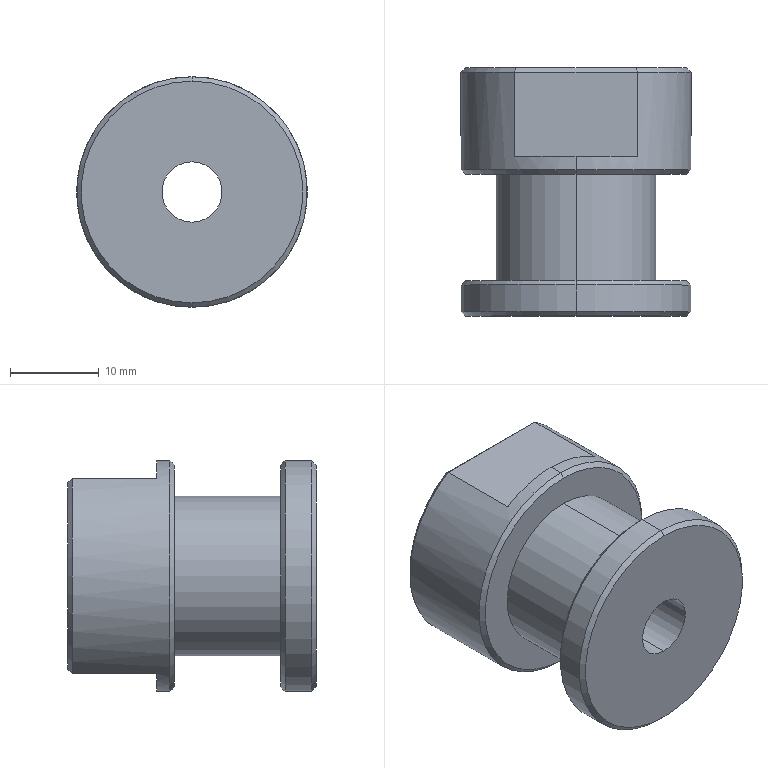Part | STEP file | 04-18 small floating joint | 1 solid | 52 faces | box 26 x 28 x 26 mm | volume 4043 mm3 | plane 20 | cone 16 | cylinder 16 | commonest cylinder face diameters 24.84 x4 26 x4 6.8 x2 12.16 x2 16.84 x2 18 x2
STEP:
#1=CARTESIAN_POINT('',(0.,-16.,-12.5));
#2=VERTEX_POINT('',#1);
#3=CARTESIAN_POINT('',(0.,-16.,12.5));
#4=VERTEX_POINT('',#3);
#5=CARTESIAN_POINT('',(0.,-16.,0.));
#6=DIRECTION('',(0.,-1.,0.));
#7=DIRECTION('',(0.,0.,-1.));
#8=AXIS2_PLACEMENT_3D('',#5,#6,#7);
#9=CIRCLE('',#8,12.5);
#10=EDGE_CURVE('',#2,#4,#9,.T.);
#11=ORIENTED_EDGE('',*,*,#10,.F.);
#12=CARTESIAN_POINT('',(0.,-15.5,-13.));
#13=VERTEX_POINT('',#12);
#14=CARTESIAN_POINT('',(0.,-16.,-12.5));
#15=DIRECTION('',(0.,0.7071,-0.7071));
#16=VECTOR('',#15,1000.);
#17=LINE('',#14,#16);
#18=EDGE_CURVE('',#2,#13,#17,.T.);
#19=ORIENTED_EDGE('',*,*,#18,.T.);
#20=CARTESIAN_POINT('',(0.,-15.5,13.));
#21=VERTEX_POINT('',#20);
#22=CARTESIAN_POINT('',(0.,-15.5,0.));
#23=DIRECTION('',(0.,1.,0.));
#24=DIRECTION('',(0.,0.,-1.));
#25=AXIS2_PLACEMENT_3D('',#22,#23,#24);
#26=CIRCLE('',#25,13.);
#27=EDGE_CURVE('',#21,#13,#26,.T.);
#28=ORIENTED_EDGE('',*,*,#27,.F.);
#29=CARTESIAN_POINT('',(0.,-16.,12.5));
#30=DIRECTION('',(0.,0.7071,0.7071));
#31=VECTOR('',#30,1000.);
#32=LINE('',#29,#31);
#33=EDGE_CURVE('',#4,#21,#32,.T.);
#34=ORIENTED_EDGE('',*,*,#33,.F.);
#35=EDGE_LOOP('',(#11,#19,#28,#34));
#36=FACE_OUTER_BOUND('',#35,.T.);
#37=CARTESIAN_POINT('',(0.,-16.,0.));
#38=DIRECTION('',(0.,1.,0.));
#39=DIRECTION('',(0.,0.,1.));
#40=AXIS2_PLACEMENT_3D('',#37,#38,#39);
#41=CONICAL_SURFACE('',#40,12.5,0.7854);
#42=ADVANCED_FACE('',(#36),#41,.T.);
#43=CARTESIAN_POINT('',(0.,0.,-12.5));
#44=VERTEX_POINT('',#43);
#45=CARTESIAN_POINT('',(0.,0.,12.5));
#46=VERTEX_POINT('',#45);
#47=CARTESIAN_POINT('',(0.,0.,0.));
#48=DIRECTION('',(0.,-1.,0.));
#49=DIRECTION('',(0.,0.,-1.));
#50=AXIS2_PLACEMENT_3D('',#47,#48,#49);
#51=CIRCLE('',#50,12.5);
#52=EDGE_CURVE('',#44,#46,#51,.T.);
#53=ORIENTED_EDGE('',*,*,#52,.F.);
#54=CARTESIAN_POINT('',(0.,0.5,-13.));
#55=VERTEX_POINT('',#54);
#56=CARTESIAN_POINT('',(0.,0.,-12.5));
#57=DIRECTION('',(0.,0.7071,-0.7071));
#58=VECTOR('',#57,1000.);
#59=LINE('',#56,#58);
#60=EDGE_CURVE('',#44,#55,#59,.T.);
#61=ORIENTED_EDGE('',*,*,#60,.T.);
#62=CARTESIAN_POINT('',(0.,0.5,13.));
#63=VERTEX_POINT('',#62);
#64=CARTESIAN_POINT('',(0.,0.5,0.));
#65=DIRECTION('',(0.,1.,0.));
#66=DIRECTION('',(0.,0.,-1.));
#67=AXIS2_PLACEMENT_3D('',#64,#65,#66);
#68=CIRCLE('',#67,13.);
#69=EDGE_CURVE('',#63,#55,#68,.T.);
#70=ORIENTED_EDGE('',*,*,#69,.F.);
#71=CARTESIAN_POINT('',(0.,0.,12.5));
#72=DIRECTION('',(0.,0.7071,0.7071));
#73=VECTOR('',#72,1000.);
#74=LINE('',#71,#73);
#75=EDGE_CURVE('',#46,#63,#74,.T.);
#76=ORIENTED_EDGE('',*,*,#75,.F.);
#77=EDGE_LOOP('',(#53,#61,#70,#76));
#78=FACE_OUTER_BOUND('',#77,.T.);
#79=CARTESIAN_POINT('',(0.,0.,0.));
#80=DIRECTION('',(0.,1.,0.));
#81=DIRECTION('',(0.,0.,1.));
#82=AXIS2_PLACEMENT_3D('',#79,#80,#81);
#83=CONICAL_SURFACE('',#82,12.5,0.7854);
#84=ADVANCED_FACE('',(#78),#83,.T.);
#85=CARTESIAN_POINT('',(0.,-12.,12.5));
#86=VERTEX_POINT('',#85);
#87=CARTESIAN_POINT('',(0.,-12.,-12.5));
#88=VERTEX_POINT('',#87);
#89=CARTESIAN_POINT('',(0.,-12.,0.));
#90=DIRECTION('',(0.,1.,0.));
#91=DIRECTION('',(0.,0.,1.));
#92=AXIS2_PLACEMENT_3D('',#89,#90,#91);
#93=CIRCLE('',#92,12.5);
#94=EDGE_CURVE('',#86,#88,#93,.T.);
#95=ORIENTED_EDGE('',*,*,#94,.F.);
#96=CARTESIAN_POINT('',(0.,-12.5,13.));
#97=VERTEX_POINT('',#96);
#98=CARTESIAN_POINT('',(0.,-12.5,13.));
#99=DIRECTION('',(0.,-0.7071,0.7071));
#100=VECTOR('',#99,1000.);
#101=LINE('',#98,#100);
#102=EDGE_CURVE('',#86,#97,#101,.T.);
#103=ORIENTED_EDGE('',*,*,#102,.T.);
#104=CARTESIAN_POINT('',(0.,-12.5,-13.));
#105=VERTEX_POINT('',#104);
#106=CARTESIAN_POINT('',(0.,-12.5,0.));
#107=DIRECTION('',(0.,-1.,0.));
#108=DIRECTION('',(0.,0.,1.));
#109=AXIS2_PLACEMENT_3D('',#106,#107,#108);
#110=CIRCLE('',#109,13.);
#111=EDGE_CURVE('',#105,#97,#110,.T.);
#112=ORIENTED_EDGE('',*,*,#111,.F.);
#113=CARTESIAN_POINT('',(0.,-12.5,-13.));
#114=DIRECTION('',(0.,-0.7071,-0.7071));
#115=VECTOR('',#114,1000.);
#116=LINE('',#113,#115);
#117=EDGE_CURVE('',#88,#105,#116,.T.);
#118=ORIENTED_EDGE('',*,*,#117,.F.);
#119=EDGE_LOOP('',(#95,#103,#112,#118));
#120=FACE_OUTER_BOUND('',#119,.T.);
#121=CARTESIAN_POINT('',(0.,-12.5,0.));
#122=DIRECTION('',(0.,-1.,0.));
#123=DIRECTION('',(0.,0.,-1.));
#124=AXIS2_PLACEMENT_3D('',#121,#122,#123);
#125=CONICAL_SURFACE('',#124,13.,0.7854);
#126=ADVANCED_FACE('',(#120),#125,.T.);
#127=CARTESIAN_POINT('',(0.,12.,3.4));
#128=VERTEX_POINT('',#127);
#129=CARTESIAN_POINT('',(0.,12.,-3.4));
#130=VERTEX_POINT('',#129);
#131=CARTESIAN_POINT('',(0.,12.,0.));
#132=DIRECTION('',(0.,-1.,0.));
#133=DIRECTION('',(0.,0.,-1.));
#134=AXIS2_PLACEMENT_3D('',#131,#132,#133);
#135=CIRCLE('',#134,3.4);
#136=EDGE_CURVE('',#128,#130,#135,.T.);
#137=ORIENTED_EDGE('',*,*,#136,.F.);
#138=CARTESIAN_POINT('',(0.,-16.,3.4));
#139=VERTEX_POINT('',#138);
#140=CARTESIAN_POINT('',(0.,-16.,3.4));
#141=DIRECTION('',(0.,-1.,0.));
#142=VECTOR('',#141,1000.);
#143=LINE('',#140,#142);
#144=EDGE_CURVE('',#128,#139,#143,.T.);
#145=ORIENTED_EDGE('',*,*,#144,.T.);
#146=CARTESIAN_POINT('',(0.,-16.,-3.4));
#147=VERTEX_POINT('',#146);
#148=CARTESIAN_POINT('',(0.,-16.,0.));
#149=DIRECTION('',(0.,-1.,0.));
#150=DIRECTION('',(0.,0.,-1.));
#151=AXIS2_PLACEMENT_3D('',#148,#149,#150);
#152=CIRCLE('',#151,3.4);
#153=EDGE_CURVE('',#139,#147,#152,.T.);
#154=ORIENTED_EDGE('',*,*,#153,.T.);
#155=CARTESIAN_POINT('',(0.,-16.,-3.4));
#156=DIRECTION('',(0.,-1.,0.));
#157=VECTOR('',#156,1000.);
#158=LINE('',#155,#157);
#159=EDGE_CURVE('',#130,#147,#158,.T.);
#160=ORIENTED_EDGE('',*,*,#159,.F.);
#161=EDGE_LOOP('',(#137,#145,#154,#160));
#162=FACE_OUTER_BOUND('',#161,.T.);
#163=CARTESIAN_POINT('',(0.,-16.,0.));
#164=DIRECTION('',(0.,-1.,0.));
#165=DIRECTION('',(0.,0.,-1.));
#166=AXIS2_PLACEMENT_3D('',#163,#164,#165);
#167=CYLINDRICAL_SURFACE('',#166,3.4);
#168=ADVANCED_FACE('',(#162),#167,.F.);
#169=CARTESIAN_POINT('',(0.,0.,-9.));
#170=VERTEX_POINT('',#169);
#171=CARTESIAN_POINT('',(0.,0.,9.));
#172=VERTEX_POINT('',#171);
#173=CARTESIAN_POINT('',(0.,0.,0.));
#174=DIRECTION('',(0.,-1.,0.));
#175=DIRECTION('',(0.,0.,-1.));
#176=AXIS2_PLACEMENT_3D('',#173,#174,#175);
#177=CIRCLE('',#176,9.);
#178=EDGE_CURVE('',#170,#172,#177,.T.);
#179=ORIENTED_EDGE('',*,*,#178,.T.);
#180=CARTESIAN_POINT('',(0.,-12.,9.));
#181=VERTEX_POINT('',#180);
#182=CARTESIAN_POINT('',(0.,12.,9.));
#183=DIRECTION('',(0.,-1.,0.));
#184=VECTOR('',#183,1000.);
#185=LINE('',#182,#184);
#186=EDGE_CURVE('',#172,#181,#185,.T.);
#187=ORIENTED_EDGE('',*,*,#186,.T.);
#188=CARTESIAN_POINT('',(0.,-12.,-9.));
#189=VERTEX_POINT('',#188);
#190=CARTESIAN_POINT('',(0.,-12.,0.));
#191=DIRECTION('',(0.,-1.,0.));
#192=DIRECTION('',(0.,0.,-1.));
#193=AXIS2_PLACEMENT_3D('',#190,#191,#192);
#194=CIRCLE('',#193,9.);
#195=EDGE_CURVE('',#189,#181,#194,.T.);
#196=ORIENTED_EDGE('',*,*,#195,.F.);
#197=CARTESIAN_POINT('',(0.,12.,-9.));
#198=DIRECTION('',(0.,-1.,0.));
#199=VECTOR('',#198,1000.);
#200=LINE('',#197,#199);
#201=EDGE_CURVE('',#170,#189,#200,.T.);
#202=ORIENTED_EDGE('',*,*,#201,.F.);
#203=EDGE_LOOP('',(#179,#187,#196,#202));
#204=FACE_OUTER_BOUND('',#203,.T.);
#205=CARTESIAN_POINT('',(0.,12.,0.));
#206=DIRECTION('',(0.,-1.,0.));
#207=DIRECTION('',(0.,0.,-1.));
#208=AXIS2_PLACEMENT_3D('',#205,#206,#207);
#209=CYLINDRICAL_SURFACE('',#208,9.);
#210=ADVANCED_FACE('',(#204),#209,.T.);
#211=ORIENTED_EDGE('',*,*,#111,.T.);
#212=CARTESIAN_POINT('',(0.,12.,13.));
#213=DIRECTION('',(0.,-1.,0.));
#214=VECTOR('',#213,1000.);
#215=LINE('',#212,#214);
#216=EDGE_CURVE('',#97,#21,#215,.T.);
#217=ORIENTED_EDGE('',*,*,#216,.T.);
#218=ORIENTED_EDGE('',*,*,#27,.T.);
#219=CARTESIAN_POINT('',(0.,12.,-13.));
#220=DIRECTION('',(0.,-1.,0.));
#221=VECTOR('',#220,1000.);
#222=LINE('',#219,#221);
#223=EDGE_CURVE('',#105,#13,#222,.T.);
#224=ORIENTED_EDGE('',*,*,#223,.F.);
#225=EDGE_LOOP('',(#211,#217,#218,#224));
#226=FACE_OUTER_BOUND('',#225,.T.);
#227=CARTESIAN_POINT('',(0.,12.,0.));
#228=DIRECTION('',(0.,-1.,0.));
#229=DIRECTION('',(0.,0.,-1.));
#230=AXIS2_PLACEMENT_3D('',#227,#228,#229);
#231=CYLINDRICAL_SURFACE('',#230,13.);
#232=ADVANCED_FACE('',(#226),#231,.T.);
#233=CARTESIAN_POINT('',(0.,2.,13.));
#234=VERTEX_POINT('',#233);
#235=CARTESIAN_POINT('',(6.928,2.,11.));
#236=VERTEX_POINT('',#235);
#237=CARTESIAN_POINT('',(0.,2.,0.));
#238=DIRECTION('',(0.,1.,0.));
#239=DIRECTION('',(0.,0.,1.));
#240=AXIS2_PLACEMENT_3D('',#237,#238,#239);
#241=CIRCLE('',#240,13.);
#242=EDGE_CURVE('',#234,#236,#241,.T.);
#243=ORIENTED_EDGE('',*,*,#242,.F.);
#244=CARTESIAN_POINT('',(0.,12.,13.));
#245=DIRECTION('',(0.,-1.,0.));
#246=VECTOR('',#245,1000.);
#247=LINE('',#244,#246);
#248=EDGE_CURVE('',#234,#63,#247,.T.);
#249=ORIENTED_EDGE('',*,*,#248,.T.);
#250=ORIENTED_EDGE('',*,*,#69,.T.);
#251=CARTESIAN_POINT('',(0.,2.,-13.));
#252=VERTEX_POINT('',#251);
#253=CARTESIAN_POINT('',(0.,12.,-13.));
#254=DIRECTION('',(0.,-1.,0.));
#255=VECTOR('',#254,1000.);
#256=LINE('',#253,#255);
#257=EDGE_CURVE('',#252,#55,#256,.T.);
#258=ORIENTED_EDGE('',*,*,#257,.F.);
#259=CARTESIAN_POINT('',(6.928,2.,-11.));
#260=VERTEX_POINT('',#259);
#261=CARTESIAN_POINT('',(0.,2.,0.));
#262=DIRECTION('',(0.,1.,0.));
#263=DIRECTION('',(0.,0.,1.));
#264=AXIS2_PLACEMENT_3D('',#261,#262,#263);
#265=CIRCLE('',#264,13.);
#266=EDGE_CURVE('',#260,#252,#265,.T.);
#267=ORIENTED_EDGE('',*,*,#266,.F.);
#268=CARTESIAN_POINT('',(6.928,11.5,-11.));
#269=VERTEX_POINT('',#268);
#270=CARTESIAN_POINT('',(6.928,2.,-11.));
#271=DIRECTION('',(0.,1.,0.));
#272=VECTOR('',#271,1000.);
#273=LINE('',#270,#272);
#274=EDGE_CURVE('',#260,#269,#273,.T.);
#275=ORIENTED_EDGE('',*,*,#274,.T.);
#276=CARTESIAN_POINT('',(6.928,11.5,11.));
#277=VERTEX_POINT('',#276);
#278=CARTESIAN_POINT('',(0.,11.5,0.));
#279=DIRECTION('',(0.,-1.,0.));
#280=DIRECTION('',(0.,0.,1.));
#281=AXIS2_PLACEMENT_3D('',#278,#279,#280);
#282=CIRCLE('',#281,13.);
#283=EDGE_CURVE('',#269,#277,#282,.T.);
#284=ORIENTED_EDGE('',*,*,#283,.T.);
#285=CARTESIAN_POINT('',(6.928,2.,11.));
#286=DIRECTION('',(0.,1.,0.));
#287=VECTOR('',#286,1000.);
#288=LINE('',#285,#287);
#289=EDGE_CURVE('',#236,#277,#288,.T.);
#290=ORIENTED_EDGE('',*,*,#289,.F.);
#291=EDGE_LOOP('',(#243,#249,#250,#258,#267,#275,#284,#290));
#292=FACE_OUTER_BOUND('',#291,.T.);
#293=CARTESIAN_POINT('',(0.,12.,0.));
#294=DIRECTION('',(0.,-1.,0.));
#295=DIRECTION('',(0.,0.,-1.));
#296=AXIS2_PLACEMENT_3D('',#293,#294,#295);
#297=CYLINDRICAL_SURFACE('',#296,13.);
#298=ADVANCED_FACE('',(#292),#297,.T.);
#299=ORIENTED_EDGE('',*,*,#248,.F.);
#300=CARTESIAN_POINT('',(-6.928,2.,11.));
#301=VERTEX_POINT('',#300);
#302=CARTESIAN_POINT('',(0.,2.,0.));
#303=DIRECTION('',(0.,1.,0.));
#304=DIRECTION('',(0.,0.,1.));
#305=AXIS2_PLACEMENT_3D('',#302,#303,#304);
#306=CIRCLE('',#305,13.);
#307=EDGE_CURVE('',#301,#234,#306,.T.);
#308=ORIENTED_EDGE('',*,*,#307,.F.);
#309=CARTESIAN_POINT('',(-6.928,11.5,11.));
#310=VERTEX_POINT('',#309);
#311=CARTESIAN_POINT('',(-6.928,2.,11.));
#312=DIRECTION('',(0.,1.,0.));
#313=VECTOR('',#312,1000.);
#314=LINE('',#311,#313);
#315=EDGE_CURVE('',#301,#310,#314,.T.);
#316=ORIENTED_EDGE('',*,*,#315,.T.);
#317=CARTESIAN_POINT('',(-6.928,11.5,-11.));
#318=VERTEX_POINT('',#317);
#319=CARTESIAN_POINT('',(0.,11.5,0.));
#320=DIRECTION('',(0.,-1.,0.));
#321=DIRECTION('',(0.,0.,1.));
#322=AXIS2_PLACEMENT_3D('',#319,#320,#321);
#323=CIRCLE('',#322,13.);
#324=EDGE_CURVE('',#310,#318,#323,.T.);
#325=ORIENTED_EDGE('',*,*,#324,.T.);
#326=CARTESIAN_POINT('',(-6.928,2.,-11.));
#327=VERTEX_POINT('',#326);
#328=CARTESIAN_POINT('',(-6.928,2.,-11.));
#329=DIRECTION('',(0.,1.,0.));
#330=VECTOR('',#329,1000.);
#331=LINE('',#328,#330);
#332=EDGE_CURVE('',#327,#318,#331,.T.);
#333=ORIENTED_EDGE('',*,*,#332,.F.);
#334=CARTESIAN_POINT('',(0.,2.,0.));
#335=DIRECTION('',(0.,1.,0.));
#336=DIRECTION('',(0.,0.,1.));
#337=AXIS2_PLACEMENT_3D('',#334,#335,#336);
#338=CIRCLE('',#337,13.);
#339=EDGE_CURVE('',#252,#327,#338,.T.);
#340=ORIENTED_EDGE('',*,*,#339,.F.);
#341=ORIENTED_EDGE('',*,*,#257,.T.);
#342=CARTESIAN_POINT('',(0.,0.5,0.));
#343=DIRECTION('',(0.,1.,0.));
#344=DIRECTION('',(0.,0.,-1.));
#345=AXIS2_PLACEMENT_3D('',#342,#343,#344);
#346=CIRCLE('',#345,13.);
#347=EDGE_CURVE('',#55,#63,#346,.T.);
#348=ORIENTED_EDGE('',*,*,#347,.T.);
#349=EDGE_LOOP('',(#299,#308,#316,#325,#333,#340,#341,#348));
#350=FACE_OUTER_BOUND('',#349,.T.);
#351=CARTESIAN_POINT('',(0.,12.,0.));
#352=DIRECTION('',(0.,-1.,0.));
#353=DIRECTION('',(0.,0.,-1.));
#354=AXIS2_PLACEMENT_3D('',#351,#352,#353);
#355=CYLINDRICAL_SURFACE('',#354,13.);
#356=ADVANCED_FACE('',(#350),#355,.T.);
#357=CARTESIAN_POINT('',(-6.782,12.,10.5));
#358=VERTEX_POINT('',#357);
#359=CARTESIAN_POINT('',(6.782,12.,10.5));
#360=VERTEX_POINT('',#359);
#361=CARTESIAN_POINT('',(6.928,12.,10.5));
#362=DIRECTION('',(1.,0.,0.));
#363=VECTOR('',#362,1000.);
#364=LINE('',#361,#363);
#365=EDGE_CURVE('',#358,#360,#364,.T.);
#366=ORIENTED_EDGE('',*,*,#365,.T.);
#367=CARTESIAN_POINT('',(6.782,12.,-10.5));
#368=VERTEX_POINT('',#367);
#369=CARTESIAN_POINT('',(0.,12.,0.));
#370=DIRECTION('',(0.,1.,0.));
#371=DIRECTION('',(0.,0.,1.));
#372=AXIS2_PLACEMENT_3D('',#369,#370,#371);
#373=CIRCLE('',#372,12.5);
#374=EDGE_CURVE('',#360,#368,#373,.T.);
#375=ORIENTED_EDGE('',*,*,#374,.T.);
#376=CARTESIAN_POINT('',(-6.782,12.,-10.5));
#377=VERTEX_POINT('',#376);
#378=CARTESIAN_POINT('',(-6.928,12.,-10.5));
#379=DIRECTION('',(-1.,0.,0.));
#380=VECTOR('',#379,1000.);
#381=LINE('',#378,#380);
#382=EDGE_CURVE('',#368,#377,#381,.T.);
#383=ORIENTED_EDGE('',*,*,#382,.T.);
#384=CARTESIAN_POINT('',(0.,12.,0.));
#385=DIRECTION('',(0.,1.,0.));
#386=DIRECTION('',(0.,0.,1.));
#387=AXIS2_PLACEMENT_3D('',#384,#385,#386);
#388=CIRCLE('',#387,12.5);
#389=EDGE_CURVE('',#377,#358,#388,.T.);
#390=ORIENTED_EDGE('',*,*,#389,.T.);
#391=EDGE_LOOP('',(#366,#375,#383,#390));
#392=FACE_OUTER_BOUND('',#391,.T.);
#393=CARTESIAN_POINT('',(0.,12.,0.));
#394=DIRECTION('',(0.,-1.,0.));
#395=DIRECTION('',(0.,0.,-1.));
#396=AXIS2_PLACEMENT_3D('',#393,#394,#395);
#397=CIRCLE('',#396,3.4);
#398=EDGE_CURVE('',#130,#128,#397,.T.);
#399=ORIENTED_EDGE('',*,*,#398,.T.);
#400=ORIENTED_EDGE('',*,*,#136,.T.);
#401=EDGE_LOOP('',(#399,#400));
#402=FACE_BOUND('',#401,.T.);
#403=CARTESIAN_POINT('',(13.,12.,0.));
#404=DIRECTION('',(0.,1.,0.));
#405=DIRECTION('',(0.,0.,1.));
#406=AXIS2_PLACEMENT_3D('',#403,#404,#405);
#407=PLANE('',#406);
#408=ADVANCED_FACE('',(#392,#402),#407,.T.);
#409=CARTESIAN_POINT('',(0.,-16.,0.));
#410=DIRECTION('',(0.,-1.,0.));
#411=DIRECTION('',(0.,0.,-1.));
#412=AXIS2_PLACEMENT_3D('',#409,#410,#411);
#413=CIRCLE('',#412,12.5);
#414=EDGE_CURVE('',#4,#2,#413,.T.);
#415=ORIENTED_EDGE('',*,*,#414,.T.);
#416=ORIENTED_EDGE('',*,*,#10,.T.);
#417=EDGE_LOOP('',(#415,#416));
#418=FACE_OUTER_BOUND('',#417,.T.);
#419=CARTESIAN_POINT('',(0.,-16.,0.));
#420=DIRECTION('',(0.,-1.,0.));
#421=DIRECTION('',(0.,0.,-1.));
#422=AXIS2_PLACEMENT_3D('',#419,#420,#421);
#423=CIRCLE('',#422,3.4);
#424=EDGE_CURVE('',#147,#139,#423,.T.);
#425=ORIENTED_EDGE('',*,*,#424,.F.);
#426=ORIENTED_EDGE('',*,*,#153,.F.);
#427=EDGE_LOOP('',(#425,#426));
#428=FACE_BOUND('',#427,.T.);
#429=CARTESIAN_POINT('',(0.,-16.,0.));
#430=DIRECTION('',(0.,-1.,0.));
#431=DIRECTION('',(0.,0.,-1.));
#432=AXIS2_PLACEMENT_3D('',#429,#430,#431);
#433=PLANE('',#432);
#434=ADVANCED_FACE('',(#418,#428),#433,.T.);
#435=ORIENTED_EDGE('',*,*,#216,.F.);
#436=CARTESIAN_POINT('',(0.,-12.5,0.));
#437=DIRECTION('',(0.,-1.,0.));
#438=DIRECTION('',(0.,0.,1.));
#439=AXIS2_PLACEMENT_3D('',#436,#437,#438);
#440=CIRCLE('',#439,13.);
#441=EDGE_CURVE('',#97,#105,#440,.T.);
#442=ORIENTED_EDGE('',*,*,#441,.T.);
#443=ORIENTED_EDGE('',*,*,#223,.T.);
#444=CARTESIAN_POINT('',(0.,-15.5,0.));
#445=DIRECTION('',(0.,1.,0.));
#446=DIRECTION('',(0.,0.,-1.));
#447=AXIS2_PLACEMENT_3D('',#444,#445,#446);
#448=CIRCLE('',#447,13.);
#449=EDGE_CURVE('',#13,#21,#448,.T.);
#450=ORIENTED_EDGE('',*,*,#449,.T.);
#451=EDGE_LOOP('',(#435,#442,#443,#450));
#452=FACE_OUTER_BOUND('',#451,.T.);
#453=CARTESIAN_POINT('',(0.,12.,0.));
#454=DIRECTION('',(0.,-1.,0.));
#455=DIRECTION('',(0.,0.,-1.));
#456=AXIS2_PLACEMENT_3D('',#453,#454,#455);
#457=CYLINDRICAL_SURFACE('',#456,13.);
#458=ADVANCED_FACE('',(#452),#457,.T.);
#459=CARTESIAN_POINT('',(0.,-12.,0.));
#460=DIRECTION('',(0.,1.,0.));
#461=DIRECTION('',(0.,0.,1.));
#462=AXIS2_PLACEMENT_3D('',#459,#460,#461);
#463=CIRCLE('',#462,12.5);
#464=EDGE_CURVE('',#88,#86,#463,.T.);
#465=ORIENTED_EDGE('',*,*,#464,.T.);
#466=ORIENTED_EDGE('',*,*,#94,.T.);
#467=EDGE_LOOP('',(#465,#466));
#468=FACE_OUTER_BOUND('',#467,.T.);
#469=ORIENTED_EDGE('',*,*,#195,.T.);
#470=CARTESIAN_POINT('',(0.,-12.,0.));
#471=DIRECTION('',(0.,-1.,0.));
#472=DIRECTION('',(0.,0.,-1.));
#473=AXIS2_PLACEMENT_3D('',#470,#471,#472);
#474=CIRCLE('',#473,9.);
#475=EDGE_CURVE('',#181,#189,#474,.T.);
#476=ORIENTED_EDGE('',*,*,#475,.T.);
#477=EDGE_LOOP('',(#469,#476));
#478=FACE_BOUND('',#477,.T.);
#479=CARTESIAN_POINT('',(13.,-12.,0.));
#480=DIRECTION('',(0.,1.,0.));
#481=DIRECTION('',(0.,0.,1.));
#482=AXIS2_PLACEMENT_3D('',#479,#480,#481);
#483=PLANE('',#482);
#484=ADVANCED_FACE('',(#468,#478),#483,.T.);
#485=ORIENTED_EDGE('',*,*,#186,.F.);
#486=CARTESIAN_POINT('',(0.,0.,0.));
#487=DIRECTION('',(0.,-1.,0.));
#488=DIRECTION('',(0.,0.,-1.));
#489=AXIS2_PLACEMENT_3D('',#486,#487,#488);
#490=CIRCLE('',#489,9.);
#491=EDGE_CURVE('',#172,#170,#490,.T.);
#492=ORIENTED_EDGE('',*,*,#491,.T.);
#493=ORIENTED_EDGE('',*,*,#201,.T.);
#494=ORIENTED_EDGE('',*,*,#475,.F.);
#495=EDGE_LOOP('',(#485,#492,#493,#494));
#496=FACE_OUTER_BOUND('',#495,.T.);
#497=CARTESIAN_POINT('',(0.,12.,0.));
#498=DIRECTION('',(0.,-1.,0.));
#499=DIRECTION('',(0.,0.,-1.));
#500=AXIS2_PLACEMENT_3D('',#497,#498,#499);
#501=CYLINDRICAL_SURFACE('',#500,9.);
#502=ADVANCED_FACE('',(#496),#501,.T.);
#503=CARTESIAN_POINT('',(0.,0.,0.));
#504=DIRECTION('',(0.,-1.,0.));
#505=DIRECTION('',(0.,0.,-1.));
#506=AXIS2_PLACEMENT_3D('',#503,#504,#505);
#507=CIRCLE('',#506,12.5);
#508=EDGE_CURVE('',#46,#44,#507,.T.);
#509=ORIENTED_EDGE('',*,*,#508,.T.);
#510=ORIENTED_EDGE('',*,*,#52,.T.);
#511=EDGE_LOOP('',(#509,#510));
#512=FACE_OUTER_BOUND('',#511,.T.);
#513=ORIENTED_EDGE('',*,*,#178,.F.);
#514=ORIENTED_EDGE('',*,*,#491,.F.);
#515=EDGE_LOOP('',(#513,#514));
#516=FACE_BOUND('',#515,.T.);
#517=CARTESIAN_POINT('',(9.,0.,0.));
#518=DIRECTION('',(0.,-1.,0.));
#519=DIRECTION('',(0.,0.,-1.));
#520=AXIS2_PLACEMENT_3D('',#517,#518,#519);
#521=PLANE('',#520);
#522=ADVANCED_FACE('',(#512,#516),#521,.T.);
#523=ORIENTED_EDGE('',*,*,#332,.T.);
#524=CARTESIAN_POINT('',(6.928,11.5,-11.));
#525=DIRECTION('',(1.,0.,0.));
#526=VECTOR('',#525,1000.);
#527=LINE('',#524,#526);
#528=EDGE_CURVE('',#318,#269,#527,.T.);
#529=ORIENTED_EDGE('',*,*,#528,.T.);
#530=ORIENTED_EDGE('',*,*,#274,.F.);
#531=CARTESIAN_POINT('',(-6.928,2.,-11.));
#532=DIRECTION('',(1.,0.,0.));
#533=VECTOR('',#532,1000.);
#534=LINE('',#531,#533);
#535=EDGE_CURVE('',#327,#260,#534,.T.);
#536=ORIENTED_EDGE('',*,*,#535,.F.);
#537=EDGE_LOOP('',(#523,#529,#530,#536));
#538=FACE_OUTER_BOUND('',#537,.T.);
#539=CARTESIAN_POINT('',(-6.928,2.,-11.));
#540=DIRECTION('',(0.,0.,1.));
#541=DIRECTION('',(1.,0.,0.));
#542=AXIS2_PLACEMENT_3D('',#539,#540,#541);
#543=PLANE('',#542);
#544=ADVANCED_FACE('',(#538),#543,.F.);
#545=ORIENTED_EDGE('',*,*,#266,.T.);
#546=ORIENTED_EDGE('',*,*,#339,.T.);
#547=ORIENTED_EDGE('',*,*,#535,.T.);
#548=EDGE_LOOP('',(#545,#546,#547));
#549=FACE_OUTER_BOUND('',#548,.T.);
#550=CARTESIAN_POINT('',(0.,2.,0.));
#551=DIRECTION('',(0.,1.,0.));
#552=DIRECTION('',(0.,0.,1.));
#553=AXIS2_PLACEMENT_3D('',#550,#551,#552);
#554=PLANE('',#553);
#555=ADVANCED_FACE('',(#549),#554,.T.);
#556=ORIENTED_EDGE('',*,*,#289,.T.);
#557=CARTESIAN_POINT('',(-6.928,11.5,11.));
#558=DIRECTION('',(-1.,0.,0.));
#559=VECTOR('',#558,1000.);
#560=LINE('',#557,#559);
#561=EDGE_CURVE('',#277,#310,#560,.T.);
#562=ORIENTED_EDGE('',*,*,#561,.T.);
#563=ORIENTED_EDGE('',*,*,#315,.F.);
#564=CARTESIAN_POINT('',(6.928,2.,11.));
#565=DIRECTION('',(-1.,0.,0.));
#566=VECTOR('',#565,1000.);
#567=LINE('',#564,#566);
#568=EDGE_CURVE('',#236,#301,#567,.T.);
#569=ORIENTED_EDGE('',*,*,#568,.F.);
#570=EDGE_LOOP('',(#556,#562,#563,#569));
#571=FACE_OUTER_BOUND('',#570,.T.);
#572=CARTESIAN_POINT('',(6.928,2.,11.));
#573=DIRECTION('',(0.,0.,-1.));
#574=DIRECTION('',(-1.,0.,0.));
#575=AXIS2_PLACEMENT_3D('',#572,#573,#574);
#576=PLANE('',#575);
#577=ADVANCED_FACE('',(#571),#576,.F.);
#578=ORIENTED_EDGE('',*,*,#307,.T.);
#579=ORIENTED_EDGE('',*,*,#242,.T.);
#580=ORIENTED_EDGE('',*,*,#568,.T.);
#581=EDGE_LOOP('',(#578,#579,#580));
#582=FACE_OUTER_BOUND('',#581,.T.);
#583=CARTESIAN_POINT('',(0.,2.,0.));
#584=DIRECTION('',(0.,1.,0.));
#585=DIRECTION('',(0.,0.,1.));
#586=AXIS2_PLACEMENT_3D('',#583,#584,#585);
#587=PLANE('',#586);
#588=ADVANCED_FACE('',(#582),#587,.T.);
#589=ORIENTED_EDGE('',*,*,#144,.F.);
#590=ORIENTED_EDGE('',*,*,#398,.F.);
#591=ORIENTED_EDGE('',*,*,#159,.T.);
#592=ORIENTED_EDGE('',*,*,#424,.T.);
#593=EDGE_LOOP('',(#589,#590,#591,#592));
#594=FACE_OUTER_BOUND('',#593,.T.);
#595=CARTESIAN_POINT('',(0.,-16.,0.));
#596=DIRECTION('',(0.,-1.,0.));
#597=DIRECTION('',(0.,0.,-1.));
#598=AXIS2_PLACEMENT_3D('',#595,#596,#597);
#599=CYLINDRICAL_SURFACE('',#598,3.4);
#600=ADVANCED_FACE('',(#594),#599,.F.);
#601=ORIENTED_EDGE('',*,*,#102,.F.);
#602=ORIENTED_EDGE('',*,*,#464,.F.);
#603=ORIENTED_EDGE('',*,*,#117,.T.);
#604=ORIENTED_EDGE('',*,*,#441,.F.);
#605=EDGE_LOOP('',(#601,#602,#603,#604));
#606=FACE_OUTER_BOUND('',#605,.T.);
#607=CARTESIAN_POINT('',(0.,-12.5,0.));
#608=DIRECTION('',(0.,-1.,0.));
#609=DIRECTION('',(0.,0.,-1.));
#610=AXIS2_PLACEMENT_3D('',#607,#608,#609);
#611=CONICAL_SURFACE('',#610,13.,0.7854);
#612=ADVANCED_FACE('',(#606),#611,.T.);
#613=CARTESIAN_POINT('',(-6.782,12.,10.5));
#614=CARTESIAN_POINT('',(-6.831,11.833,10.667));
#615=CARTESIAN_POINT('',(-6.88,11.667,10.833));
#616=CARTESIAN_POINT('',(-6.928,11.5,11.));
#617=B_SPLINE_CURVE_WITH_KNOTS('',3,(#613,#614,#615,#616),.UNSPECIFIED.,.F.,.F.,(4,4),(0.,0.000722),.UNSPECIFIED.);
#618=EDGE_CURVE('',#358,#310,#617,.T.);
#619=ORIENTED_EDGE('',*,*,#618,.F.);
#620=ORIENTED_EDGE('',*,*,#389,.F.);
#621=CARTESIAN_POINT('',(-6.928,11.5,-11.));
#622=CARTESIAN_POINT('',(-6.88,11.667,-10.833));
#623=CARTESIAN_POINT('',(-6.831,11.833,-10.667));
#624=CARTESIAN_POINT('',(-6.782,12.,-10.5));
#625=B_SPLINE_CURVE_WITH_KNOTS('',3,(#621,#622,#623,#624),.UNSPECIFIED.,.F.,.F.,(4,4),(0.,0.000722),.UNSPECIFIED.);
#626=EDGE_CURVE('',#318,#377,#625,.T.);
#627=ORIENTED_EDGE('',*,*,#626,.F.);
#628=ORIENTED_EDGE('',*,*,#324,.F.);
#629=EDGE_LOOP('',(#619,#620,#627,#628));
#630=FACE_OUTER_BOUND('',#629,.T.);
#631=CARTESIAN_POINT('',(0.,11.5,0.));
#632=DIRECTION('',(0.,-1.,0.));
#633=DIRECTION('',(0.,0.,-1.));
#634=AXIS2_PLACEMENT_3D('',#631,#632,#633);
#635=CONICAL_SURFACE('',#634,13.,0.7854);
#636=ADVANCED_FACE('',(#630),#635,.T.);
#637=ORIENTED_EDGE('',*,*,#626,.T.);
#638=ORIENTED_EDGE('',*,*,#382,.F.);
#639=CARTESIAN_POINT('',(6.928,11.5,-11.));
#640=CARTESIAN_POINT('',(6.88,11.667,-10.833));
#641=CARTESIAN_POINT('',(6.831,11.833,-10.667));
#642=CARTESIAN_POINT('',(6.782,12.,-10.5));
#643=B_SPLINE_CURVE_WITH_KNOTS('',3,(#639,#640,#641,#642),.UNSPECIFIED.,.F.,.F.,(4,4),(0.,0.000722),.UNSPECIFIED.);
#644=EDGE_CURVE('',#269,#368,#643,.T.);
#645=ORIENTED_EDGE('',*,*,#644,.F.);
#646=ORIENTED_EDGE('',*,*,#528,.F.);
#647=EDGE_LOOP('',(#637,#638,#645,#646));
#648=FACE_OUTER_BOUND('',#647,.T.);
#649=CARTESIAN_POINT('',(-6.928,11.5,-11.));
#650=DIRECTION('',(0.,0.7071,-0.7071));
#651=DIRECTION('',(0.,0.7071,0.7071));
#652=AXIS2_PLACEMENT_3D('',#649,#650,#651);
#653=PLANE('',#652);
#654=ADVANCED_FACE('',(#648),#653,.T.);
#655=ORIENTED_EDGE('',*,*,#618,.T.);
#656=ORIENTED_EDGE('',*,*,#561,.F.);
#657=CARTESIAN_POINT('',(6.782,12.,10.5));
#658=CARTESIAN_POINT('',(6.831,11.833,10.667));
#659=CARTESIAN_POINT('',(6.88,11.667,10.833));
#660=CARTESIAN_POINT('',(6.928,11.5,11.));
#661=B_SPLINE_CURVE_WITH_KNOTS('',3,(#657,#658,#659,#660),.UNSPECIFIED.,.F.,.F.,(4,4),(0.,0.000722),.UNSPECIFIED.);
#662=EDGE_CURVE('',#360,#277,#661,.T.);
#663=ORIENTED_EDGE('',*,*,#662,.F.);
#664=ORIENTED_EDGE('',*,*,#365,.F.);
#665=EDGE_LOOP('',(#655,#656,#663,#664));
#666=FACE_OUTER_BOUND('',#665,.T.);
#667=CARTESIAN_POINT('',(6.928,11.5,11.));
#668=DIRECTION('',(0.,0.7071,0.7071));
#669=DIRECTION('',(0.,-0.7071,0.7071));
#670=AXIS2_PLACEMENT_3D('',#667,#668,#669);
#671=PLANE('',#670);
#672=ADVANCED_FACE('',(#666),#671,.T.);
#673=ORIENTED_EDGE('',*,*,#644,.T.);
#674=ORIENTED_EDGE('',*,*,#374,.F.);
#675=ORIENTED_EDGE('',*,*,#662,.T.);
#676=ORIENTED_EDGE('',*,*,#283,.F.);
#677=EDGE_LOOP('',(#673,#674,#675,#676));
#678=FACE_OUTER_BOUND('',#677,.T.);
#679=CARTESIAN_POINT('',(0.,11.5,0.));
#680=DIRECTION('',(0.,-1.,0.));
#681=DIRECTION('',(0.,0.,-1.));
#682=AXIS2_PLACEMENT_3D('',#679,#680,#681);
#683=CONICAL_SURFACE('',#682,13.,0.7854);
#684=ADVANCED_FACE('',(#678),#683,.T.);
#685=ORIENTED_EDGE('',*,*,#60,.F.);
#686=ORIENTED_EDGE('',*,*,#508,.F.);
#687=ORIENTED_EDGE('',*,*,#75,.T.);
#688=ORIENTED_EDGE('',*,*,#347,.F.);
#689=EDGE_LOOP('',(#685,#686,#687,#688));
#690=FACE_OUTER_BOUND('',#689,.T.);
#691=CARTESIAN_POINT('',(0.,0.,0.));
#692=DIRECTION('',(0.,1.,0.));
#693=DIRECTION('',(0.,0.,1.));
#694=AXIS2_PLACEMENT_3D('',#691,#692,#693);
#695=CONICAL_SURFACE('',#694,12.5,0.7854);
#696=ADVANCED_FACE('',(#690),#695,.T.);
#697=ORIENTED_EDGE('',*,*,#18,.F.);
#698=ORIENTED_EDGE('',*,*,#414,.F.);
#699=ORIENTED_EDGE('',*,*,#33,.T.);
#700=ORIENTED_EDGE('',*,*,#449,.F.);
#701=EDGE_LOOP('',(#697,#698,#699,#700));
#702=FACE_OUTER_BOUND('',#701,.T.);
#703=CARTESIAN_POINT('',(0.,-16.,0.));
#704=DIRECTION('',(0.,1.,0.));
#705=DIRECTION('',(0.,0.,1.));
#706=AXIS2_PLACEMENT_3D('',#703,#704,#705);
#707=CONICAL_SURFACE('',#706,12.5,0.7854);
#708=ADVANCED_FACE('',(#702),#707,.T.);
#709=CLOSED_SHELL('',(#42,#84,#126,#168,#210,#232,#298,#356,#408,#434,#458,#484,#502,#522,#544,#555,#577,#588,#600,#612,#636,#654,#672,#684,#696,#708));
#710=CARTESIAN_POINT('',(0.,-12.58,12.26));
#711=VERTEX_POINT('',#710);
#712=CARTESIAN_POINT('',(0.,-12.58,-12.26));
#713=VERTEX_POINT('',#712);
#714=CARTESIAN_POINT('',(0.,-12.58,0.));
#715=DIRECTION('',(0.,-1.,0.));
#716=DIRECTION('',(0.,0.,-1.));
#717=AXIS2_PLACEMENT_3D('',#714,#715,#716);
#718=CIRCLE('',#717,12.26);
#719=EDGE_CURVE('',#711,#713,#718,.T.);
#720=ORIENTED_EDGE('',*,*,#719,.F.);
#721=CARTESIAN_POINT('',(0.,-12.74,12.42));
#722=VERTEX_POINT('',#721);
#723=CARTESIAN_POINT('',(0.,-12.74,12.42));
#724=DIRECTION('',(0.,-0.7071,0.7071));
#725=VECTOR('',#724,1000.);
#726=LINE('',#723,#725);
#727=EDGE_CURVE('',#711,#722,#726,.T.);
#728=ORIENTED_EDGE('',*,*,#727,.T.);
#729=CARTESIAN_POINT('',(0.,-12.74,-12.42));
#730=VERTEX_POINT('',#729);
#731=CARTESIAN_POINT('',(0.,-12.74,0.));
#732=DIRECTION('',(0.,1.,0.));
#733=DIRECTION('',(0.,0.,-1.));
#734=AXIS2_PLACEMENT_3D('',#731,#732,#733);
#735=CIRCLE('',#734,12.42);
#736=EDGE_CURVE('',#730,#722,#735,.T.);
#737=ORIENTED_EDGE('',*,*,#736,.F.);
#738=CARTESIAN_POINT('',(0.,-12.74,-12.42));
#739=DIRECTION('',(0.,-0.7071,-0.7071));
#740=VECTOR('',#739,1000.);
#741=LINE('',#738,#740);
#742=EDGE_CURVE('',#713,#730,#741,.T.);
#743=ORIENTED_EDGE('',*,*,#742,.F.);
#744=EDGE_LOOP('',(#720,#728,#737,#743));
#745=FACE_OUTER_BOUND('',#744,.T.);
#746=CARTESIAN_POINT('',(0.,-12.74,0.));
#747=DIRECTION('',(0.,-1.,0.));
#748=DIRECTION('',(0.,0.,-1.));
#749=AXIS2_PLACEMENT_3D('',#746,#747,#748);
#750=CONICAL_SURFACE('',#749,12.42,0.7854);
#751=ADVANCED_FACE('',(#745),#750,.F.);
#752=CARTESIAN_POINT('',(0.,0.58,-12.26));
#753=VERTEX_POINT('',#752);
#754=CARTESIAN_POINT('',(0.,0.58,12.26));
#755=VERTEX_POINT('',#754);
#756=CARTESIAN_POINT('',(0.,0.58,0.));
#757=DIRECTION('',(0.,1.,0.));
#758=DIRECTION('',(0.,0.,-1.));
#759=AXIS2_PLACEMENT_3D('',#756,#757,#758);
#760=CIRCLE('',#759,12.26);
#761=EDGE_CURVE('',#753,#755,#760,.T.);
#762=ORIENTED_EDGE('',*,*,#761,.F.);
#763=CARTESIAN_POINT('',(0.,0.7402,-12.42));
#764=VERTEX_POINT('',#763);
#765=CARTESIAN_POINT('',(0.,0.58,-12.26));
#766=DIRECTION('',(0.,0.7071,-0.7071));
#767=VECTOR('',#766,1000.);
#768=LINE('',#765,#767);
#769=EDGE_CURVE('',#753,#764,#768,.T.);
#770=ORIENTED_EDGE('',*,*,#769,.T.);
#771=CARTESIAN_POINT('',(0.,0.7402,12.42));
#772=VERTEX_POINT('',#771);
#773=CARTESIAN_POINT('',(0.,0.7402,0.));
#774=DIRECTION('',(0.,-1.,0.));
#775=DIRECTION('',(0.,0.,-1.));
#776=AXIS2_PLACEMENT_3D('',#773,#774,#775);
#777=CIRCLE('',#776,12.42);
#778=EDGE_CURVE('',#772,#764,#777,.T.);
#779=ORIENTED_EDGE('',*,*,#778,.F.);
#780=CARTESIAN_POINT('',(0.,0.58,12.26));
#781=DIRECTION('',(0.,0.7071,0.7071));
#782=VECTOR('',#781,1000.);
#783=LINE('',#780,#782);
#784=EDGE_CURVE('',#755,#772,#783,.T.);
#785=ORIENTED_EDGE('',*,*,#784,.F.);
#786=EDGE_LOOP('',(#762,#770,#779,#785));
#787=FACE_OUTER_BOUND('',#786,.T.);
#788=CARTESIAN_POINT('',(0.,0.58,0.));
#789=DIRECTION('',(0.,1.,0.));
#790=DIRECTION('',(0.,0.,1.));
#791=AXIS2_PLACEMENT_3D('',#788,#789,#790);
#792=CONICAL_SURFACE('',#791,12.26,0.7854);
#793=ADVANCED_FACE('',(#787),#792,.F.);
#794=CARTESIAN_POINT('',(0.,-15.42,-12.26));
#795=VERTEX_POINT('',#794);
#796=CARTESIAN_POINT('',(0.,-15.42,12.26));
#797=VERTEX_POINT('',#796);
#798=CARTESIAN_POINT('',(0.,-15.42,0.));
#799=DIRECTION('',(0.,1.,0.));
#800=DIRECTION('',(0.,0.,-1.));
#801=AXIS2_PLACEMENT_3D('',#798,#799,#800);
#802=CIRCLE('',#801,12.26);
#803=EDGE_CURVE('',#795,#797,#802,.T.);
#804=ORIENTED_EDGE('',*,*,#803,.F.);
#805=CARTESIAN_POINT('',(0.,-15.26,-12.42));
#806=VERTEX_POINT('',#805);
#807=CARTESIAN_POINT('',(0.,-15.42,-12.26));
#808=DIRECTION('',(0.,0.7071,-0.7071));
#809=VECTOR('',#808,1000.);
#810=LINE('',#807,#809);
#811=EDGE_CURVE('',#795,#806,#810,.T.);
#812=ORIENTED_EDGE('',*,*,#811,.T.);
#813=CARTESIAN_POINT('',(0.,-15.26,12.42));
#814=VERTEX_POINT('',#813);
#815=CARTESIAN_POINT('',(0.,-15.26,0.));
#816=DIRECTION('',(0.,-1.,0.));
#817=DIRECTION('',(0.,0.,-1.));
#818=AXIS2_PLACEMENT_3D('',#815,#816,#817);
#819=CIRCLE('',#818,12.42);
#820=EDGE_CURVE('',#814,#806,#819,.T.);
#821=ORIENTED_EDGE('',*,*,#820,.F.);
#822=CARTESIAN_POINT('',(0.,-15.42,12.26));
#823=DIRECTION('',(0.,0.7071,0.7071));
#824=VECTOR('',#823,1000.);
#825=LINE('',#822,#824);
#826=EDGE_CURVE('',#797,#814,#825,.T.);
#827=ORIENTED_EDGE('',*,*,#826,.F.);
#828=EDGE_LOOP('',(#804,#812,#821,#827));
#829=FACE_OUTER_BOUND('',#828,.T.);
#830=CARTESIAN_POINT('',(0.,-15.42,0.));
#831=DIRECTION('',(0.,1.,0.));
#832=DIRECTION('',(0.,0.,1.));
#833=AXIS2_PLACEMENT_3D('',#830,#831,#832);
#834=CONICAL_SURFACE('',#833,12.26,0.7854);
#835=ADVANCED_FACE('',(#829),#834,.F.);
#836=CARTESIAN_POINT('',(0.,-15.42,6.08));
#837=VERTEX_POINT('',#836);
#838=CARTESIAN_POINT('',(0.,-15.42,-6.08));
#839=VERTEX_POINT('',#838);
#840=CARTESIAN_POINT('',(0.,-15.42,0.));
#841=DIRECTION('',(0.,1.,0.));
#842=DIRECTION('',(0.,0.,1.));
#843=AXIS2_PLACEMENT_3D('',#840,#841,#842);
#844=CIRCLE('',#843,6.08);
#845=EDGE_CURVE('',#837,#839,#844,.T.);
#846=ORIENTED_EDGE('',*,*,#845,.T.);
#847=CARTESIAN_POINT('',(0.,11.42,-6.08));
#848=VERTEX_POINT('',#847);
#849=CARTESIAN_POINT('',(0.,-15.42,-6.08));
#850=DIRECTION('',(0.,1.,0.));
#851=VECTOR('',#850,1000.);
#852=LINE('',#849,#851);
#853=EDGE_CURVE('',#839,#848,#852,.T.);
#854=ORIENTED_EDGE('',*,*,#853,.T.);
#855=CARTESIAN_POINT('',(0.,11.42,6.08));
#856=VERTEX_POINT('',#855);
#857=CARTESIAN_POINT('',(0.,11.42,0.));
#858=DIRECTION('',(0.,-1.,0.));
#859=DIRECTION('',(0.,0.,-1.));
#860=AXIS2_PLACEMENT_3D('',#857,#858,#859);
#861=CIRCLE('',#860,6.08);
#862=EDGE_CURVE('',#848,#856,#861,.T.);
#863=ORIENTED_EDGE('',*,*,#862,.T.);
#864=CARTESIAN_POINT('',(0.,-15.42,6.08));
#865=DIRECTION('',(0.,1.,0.));
#866=VECTOR('',#865,1000.);
#867=LINE('',#864,#866);
#868=EDGE_CURVE('',#837,#856,#867,.T.);
#869=ORIENTED_EDGE('',*,*,#868,.F.);
#870=EDGE_LOOP('',(#846,#854,#863,#869));
#871=FACE_OUTER_BOUND('',#870,.T.);
#872=CARTESIAN_POINT('',(0.,-15.42,0.));
#873=DIRECTION('',(0.,1.,0.));
#874=DIRECTION('',(0.,0.,1.));
#875=AXIS2_PLACEMENT_3D('',#872,#873,#874);
#876=CYLINDRICAL_SURFACE('',#875,6.08);
#877=ADVANCED_FACE('',(#871),#876,.T.);
#878=ORIENTED_EDGE('',*,*,#820,.T.);
#879=CARTESIAN_POINT('',(0.,-15.42,-12.42));
#880=DIRECTION('',(0.,1.,0.));
#881=VECTOR('',#880,1000.);
#882=LINE('',#879,#881);
#883=EDGE_CURVE('',#806,#730,#882,.T.);
#884=ORIENTED_EDGE('',*,*,#883,.T.);
#885=ORIENTED_EDGE('',*,*,#736,.T.);
#886=CARTESIAN_POINT('',(0.,-15.42,12.42));
#887=DIRECTION('',(0.,1.,0.));
#888=VECTOR('',#887,1000.);
#889=LINE('',#886,#888);
#890=EDGE_CURVE('',#814,#722,#889,.T.);
#891=ORIENTED_EDGE('',*,*,#890,.F.);
#892=EDGE_LOOP('',(#878,#884,#885,#891));
#893=FACE_OUTER_BOUND('',#892,.T.);
#894=CARTESIAN_POINT('',(0.,-15.42,0.));
#895=DIRECTION('',(0.,1.,0.));
#896=DIRECTION('',(0.,0.,1.));
#897=AXIS2_PLACEMENT_3D('',#894,#895,#896);
#898=CYLINDRICAL_SURFACE('',#897,12.42);
#899=ADVANCED_FACE('',(#893),#898,.F.);
#900=CARTESIAN_POINT('',(0.,0.58,8.42));
#901=VERTEX_POINT('',#900);
#902=CARTESIAN_POINT('',(0.,0.58,-8.42));
#903=VERTEX_POINT('',#902);
#904=CARTESIAN_POINT('',(0.,0.58,0.));
#905=DIRECTION('',(0.,-1.,0.));
#906=DIRECTION('',(0.,0.,-1.));
#907=AXIS2_PLACEMENT_3D('',#904,#905,#906);
#908=CIRCLE('',#907,8.42);
#909=EDGE_CURVE('',#901,#903,#908,.T.);
#910=ORIENTED_EDGE('',*,*,#909,.F.);
#911=CARTESIAN_POINT('',(0.,-12.58,8.42));
#912=VERTEX_POINT('',#911);
#913=CARTESIAN_POINT('',(0.,0.58,8.42));
#914=DIRECTION('',(0.,-1.,0.));
#915=VECTOR('',#914,1000.);
#916=LINE('',#913,#915);
#917=EDGE_CURVE('',#901,#912,#916,.T.);
#918=ORIENTED_EDGE('',*,*,#917,.T.);
#919=CARTESIAN_POINT('',(0.,-12.58,-8.42));
#920=VERTEX_POINT('',#919);
#921=CARTESIAN_POINT('',(0.,-12.58,0.));
#922=DIRECTION('',(0.,-1.,0.));
#923=DIRECTION('',(0.,0.,-1.));
#924=AXIS2_PLACEMENT_3D('',#921,#922,#923);
#925=CIRCLE('',#924,8.42);
#926=EDGE_CURVE('',#912,#920,#925,.T.);
#927=ORIENTED_EDGE('',*,*,#926,.T.);
#928=CARTESIAN_POINT('',(0.,0.58,-8.42));
#929=DIRECTION('',(0.,-1.,0.));
#930=VECTOR('',#929,1000.);
#931=LINE('',#928,#930);
#932=EDGE_CURVE('',#903,#920,#931,.T.);
#933=ORIENTED_EDGE('',*,*,#932,.F.);
#934=EDGE_LOOP('',(#910,#918,#927,#933));
#935=FACE_OUTER_BOUND('',#934,.T.);
#936=CARTESIAN_POINT('',(0.,0.58,0.));
#937=DIRECTION('',(0.,-1.,0.));
#938=DIRECTION('',(0.,0.,-1.));
#939=AXIS2_PLACEMENT_3D('',#936,#937,#938);
#940=CYLINDRICAL_SURFACE('',#939,8.42);
#941=ADVANCED_FACE('',(#935),#940,.F.);
#942=ORIENTED_EDGE('',*,*,#778,.T.);
#943=CARTESIAN_POINT('',(0.,1.42,-12.42));
#944=VERTEX_POINT('',#943);
#945=CARTESIAN_POINT('',(0.,0.58,-12.42));
#946=DIRECTION('',(0.,1.,0.));
#947=VECTOR('',#946,1000.);
#948=LINE('',#945,#947);
#949=EDGE_CURVE('',#764,#944,#948,.T.);
#950=ORIENTED_EDGE('',*,*,#949,.T.);
#951=CARTESIAN_POINT('',(-6.759,1.42,-10.42));
#952=VERTEX_POINT('',#951);
#953=CARTESIAN_POINT('',(0.,1.42,0.));
#954=DIRECTION('',(0.,-1.,0.));
#955=DIRECTION('',(0.,0.,1.));
#956=AXIS2_PLACEMENT_3D('',#953,#954,#955);
#957=CIRCLE('',#956,12.42);
#958=EDGE_CURVE('',#952,#944,#957,.T.);
#959=ORIENTED_EDGE('',*,*,#958,.F.);
#960=CARTESIAN_POINT('',(-6.759,11.26,-10.42));
#961=VERTEX_POINT('',#960);
#962=CARTESIAN_POINT('',(-6.759,1.42,-10.42));
#963=DIRECTION('',(0.,1.,0.));
#964=VECTOR('',#963,1000.);
#965=LINE('',#962,#964);
#966=EDGE_CURVE('',#952,#961,#965,.T.);
#967=ORIENTED_EDGE('',*,*,#966,.T.);
#968=CARTESIAN_POINT('',(-6.759,11.26,10.42));
#969=VERTEX_POINT('',#968);
#970=CARTESIAN_POINT('',(0.,11.26,0.));
#971=DIRECTION('',(0.,1.,0.));
#972=DIRECTION('',(0.,0.,-1.));
#973=AXIS2_PLACEMENT_3D('',#970,#971,#972);
#974=CIRCLE('',#973,12.42);
#975=EDGE_CURVE('',#961,#969,#974,.T.);
#976=ORIENTED_EDGE('',*,*,#975,.T.);
#977=CARTESIAN_POINT('',(-6.759,1.42,10.42));
#978=VERTEX_POINT('',#977);
#979=CARTESIAN_POINT('',(-6.759,1.42,10.42));
#980=DIRECTION('',(0.,1.,0.));
#981=VECTOR('',#980,1000.);
#982=LINE('',#979,#981);
#983=EDGE_CURVE('',#978,#969,#982,.T.);
#984=ORIENTED_EDGE('',*,*,#983,.F.);
#985=CARTESIAN_POINT('',(0.,1.42,12.42));
#986=VERTEX_POINT('',#985);
#987=CARTESIAN_POINT('',(0.,1.42,0.));
#988=DIRECTION('',(0.,-1.,0.));
#989=DIRECTION('',(0.,0.,1.));
#990=AXIS2_PLACEMENT_3D('',#987,#988,#989);
#991=CIRCLE('',#990,12.42);
#992=EDGE_CURVE('',#986,#978,#991,.T.);
#993=ORIENTED_EDGE('',*,*,#992,.F.);
#994=CARTESIAN_POINT('',(0.,0.58,12.42));
#995=DIRECTION('',(0.,1.,0.));
#996=VECTOR('',#995,1000.);
#997=LINE('',#994,#996);
#998=EDGE_CURVE('',#772,#986,#997,.T.);
#999=ORIENTED_EDGE('',*,*,#998,.F.);
#1000=EDGE_LOOP('',(#942,#950,#959,#967,#976,#984,#993,#999));
#1001=FACE_OUTER_BOUND('',#1000,.T.);
#1002=CARTESIAN_POINT('',(0.,0.58,0.));
#1003=DIRECTION('',(0.,1.,0.));
#1004=DIRECTION('',(0.,0.,1.));
#1005=AXIS2_PLACEMENT_3D('',#1002,#1003,#1004);
#1006=CYLINDRICAL_SURFACE('',#1005,12.42);
#1007=ADVANCED_FACE('',(#1001),#1006,.F.);
#1008=ORIENTED_EDGE('',*,*,#949,.F.);
#1009=CARTESIAN_POINT('',(0.,0.7402,0.));
#1010=DIRECTION('',(0.,-1.,0.));
#1011=DIRECTION('',(0.,0.,-1.));
#1012=AXIS2_PLACEMENT_3D('',#1009,#1010,#1011);
#1013=CIRCLE('',#1012,12.42);
#1014=EDGE_CURVE('',#764,#772,#1013,.T.);
#1015=ORIENTED_EDGE('',*,*,#1014,.T.);
#1016=ORIENTED_EDGE('',*,*,#998,.T.);
#1017=CARTESIAN_POINT('',(6.759,1.42,10.42));
#1018=VERTEX_POINT('',#1017);
#1019=CARTESIAN_POINT('',(0.,1.42,0.));
#1020=DIRECTION('',(0.,-1.,0.));
#1021=DIRECTION('',(0.,0.,1.));
#1022=AXIS2_PLACEMENT_3D('',#1019,#1020,#1021);
#1023=CIRCLE('',#1022,12.42);
#1024=EDGE_CURVE('',#1018,#986,#1023,.T.);
#1025=ORIENTED_EDGE('',*,*,#1024,.F.);
#1026=CARTESIAN_POINT('',(6.759,11.26,10.42));
#1027=VERTEX_POINT('',#1026);
#1028=CARTESIAN_POINT('',(6.759,1.42,10.42));
#1029=DIRECTION('',(0.,1.,0.));
#1030=VECTOR('',#1029,1000.);
#1031=LINE('',#1028,#1030);
#1032=EDGE_CURVE('',#1018,#1027,#1031,.T.);
#1033=ORIENTED_EDGE('',*,*,#1032,.T.);
#1034=CARTESIAN_POINT('',(6.759,11.26,-10.42));
#1035=VERTEX_POINT('',#1034);
#1036=CARTESIAN_POINT('',(0.,11.26,0.));
#1037=DIRECTION('',(0.,1.,0.));
#1038=DIRECTION('',(0.,0.,-1.));
#1039=AXIS2_PLACEMENT_3D('',#1036,#1037,#1038);
#1040=CIRCLE('',#1039,12.42);
#1041=EDGE_CURVE('',#1027,#1035,#1040,.T.);
#1042=ORIENTED_EDGE('',*,*,#1041,.T.);
#1043=CARTESIAN_POINT('',(6.759,1.42,-10.42));
#1044=VERTEX_POINT('',#1043);
#1045=CARTESIAN_POINT('',(6.759,1.42,-10.42));
#1046=DIRECTION('',(0.,1.,0.));
#1047=VECTOR('',#1046,1000.);
#1048=LINE('',#1045,#1047);
#1049=EDGE_CURVE('',#1044,#1035,#1048,.T.);
#1050=ORIENTED_EDGE('',*,*,#1049,.F.);
#1051=CARTESIAN_POINT('',(0.,1.42,0.));
#1052=DIRECTION('',(0.,-1.,0.));
#1053=DIRECTION('',(0.,0.,1.));
#1054=AXIS2_PLACEMENT_3D('',#1051,#1052,#1053);
#1055=CIRCLE('',#1054,12.42);
#1056=EDGE_CURVE('',#944,#1044,#1055,.T.);
#1057=ORIENTED_EDGE('',*,*,#1056,.F.);
#1058=EDGE_LOOP('',(#1008,#1015,#1016,#1025,#1033,#1042,#1050,#1057));
#1059=FACE_OUTER_BOUND('',#1058,.T.);
#1060=CARTESIAN_POINT('',(0.,0.58,0.));
#1061=DIRECTION('',(0.,1.,0.));
#1062=DIRECTION('',(0.,0.,1.));
#1063=AXIS2_PLACEMENT_3D('',#1060,#1061,#1062);
#1064=CYLINDRICAL_SURFACE('',#1063,12.42);
#1065=ADVANCED_FACE('',(#1059),#1064,.F.);
#1066=CARTESIAN_POINT('',(6.711,11.42,-10.26));
#1067=VERTEX_POINT('',#1066);
#1068=CARTESIAN_POINT('',(6.711,11.42,10.26));
#1069=VERTEX_POINT('',#1068);
#1070=CARTESIAN_POINT('',(0.,11.42,0.));
#1071=DIRECTION('',(0.,-1.,0.));
#1072=DIRECTION('',(0.,0.,-1.));
#1073=AXIS2_PLACEMENT_3D('',#1070,#1071,#1072);
#1074=CIRCLE('',#1073,12.26);
#1075=EDGE_CURVE('',#1067,#1069,#1074,.T.);
#1076=ORIENTED_EDGE('',*,*,#1075,.T.);
#1077=CARTESIAN_POINT('',(-6.711,11.42,10.26));
#1078=VERTEX_POINT('',#1077);
#1079=CARTESIAN_POINT('',(0.,11.42,10.26));
#1080=DIRECTION('',(-1.,0.,0.));
#1081=VECTOR('',#1080,1000.);
#1082=LINE('',#1079,#1081);
#1083=EDGE_CURVE('',#1069,#1078,#1082,.T.);
#1084=ORIENTED_EDGE('',*,*,#1083,.T.);
#1085=CARTESIAN_POINT('',(-6.711,11.42,-10.26));
#1086=VERTEX_POINT('',#1085);
#1087=CARTESIAN_POINT('',(0.,11.42,0.));
#1088=DIRECTION('',(0.,-1.,0.));
#1089=DIRECTION('',(0.,0.,-1.));
#1090=AXIS2_PLACEMENT_3D('',#1087,#1088,#1089);
#1091=CIRCLE('',#1090,12.26);
#1092=EDGE_CURVE('',#1078,#1086,#1091,.T.);
#1093=ORIENTED_EDGE('',*,*,#1092,.T.);
#1094=CARTESIAN_POINT('',(0.,11.42,-10.26));
#1095=DIRECTION('',(1.,0.,0.));
#1096=VECTOR('',#1095,1000.);
#1097=LINE('',#1094,#1096);
#1098=EDGE_CURVE('',#1086,#1067,#1097,.T.);
#1099=ORIENTED_EDGE('',*,*,#1098,.T.);
#1100=EDGE_LOOP('',(#1076,#1084,#1093,#1099));
#1101=FACE_OUTER_BOUND('',#1100,.T.);
#1102=CARTESIAN_POINT('',(0.,11.42,0.));
#1103=DIRECTION('',(0.,-1.,0.));
#1104=DIRECTION('',(0.,0.,-1.));
#1105=AXIS2_PLACEMENT_3D('',#1102,#1103,#1104);
#1106=CIRCLE('',#1105,6.08);
#1107=EDGE_CURVE('',#856,#848,#1106,.T.);
#1108=ORIENTED_EDGE('',*,*,#1107,.F.);
#1109=ORIENTED_EDGE('',*,*,#862,.F.);
#1110=EDGE_LOOP('',(#1108,#1109));
#1111=FACE_BOUND('',#1110,.T.);
#1112=CARTESIAN_POINT('',(0.,11.42,0.));
#1113=DIRECTION('',(0.,-1.,0.));
#1114=DIRECTION('',(0.,0.,-1.));
#1115=AXIS2_PLACEMENT_3D('',#1112,#1113,#1114);
#1116=PLANE('',#1115);
#1117=ADVANCED_FACE('',(#1101,#1111),#1116,.T.);
#1118=CARTESIAN_POINT('',(0.,0.58,0.));
#1119=DIRECTION('',(0.,1.,0.));
#1120=DIRECTION('',(0.,0.,-1.));
#1121=AXIS2_PLACEMENT_3D('',#1118,#1119,#1120);
#1122=CIRCLE('',#1121,12.26);
#1123=EDGE_CURVE('',#755,#753,#1122,.T.);
#1124=ORIENTED_EDGE('',*,*,#1123,.T.);
#1125=ORIENTED_EDGE('',*,*,#761,.T.);
#1126=EDGE_LOOP('',(#1124,#1125));
#1127=FACE_OUTER_BOUND('',#1126,.T.);
#1128=CARTESIAN_POINT('',(0.,0.58,0.));
#1129=DIRECTION('',(0.,-1.,0.));
#1130=DIRECTION('',(0.,0.,-1.));
#1131=AXIS2_PLACEMENT_3D('',#1128,#1129,#1130);
#1132=CIRCLE('',#1131,8.42);
#1133=EDGE_CURVE('',#903,#901,#1132,.T.);
#1134=ORIENTED_EDGE('',*,*,#1133,.T.);
#1135=ORIENTED_EDGE('',*,*,#909,.T.);
#1136=EDGE_LOOP('',(#1134,#1135));
#1137=FACE_BOUND('',#1136,.T.);
#1138=CARTESIAN_POINT('',(0.,0.58,0.));
#1139=DIRECTION('',(0.,-1.,0.));
#1140=DIRECTION('',(0.,0.,-1.));
#1141=AXIS2_PLACEMENT_3D('',#1138,#1139,#1140);
#1142=PLANE('',#1141);
#1143=ADVANCED_FACE('',(#1127,#1137),#1142,.F.);
#1144=ORIENTED_EDGE('',*,*,#1049,.T.);
#1145=CARTESIAN_POINT('',(-6.759,11.26,-10.42));
#1146=DIRECTION('',(-1.,0.,0.));
#1147=VECTOR('',#1146,1000.);
#1148=LINE('',#1145,#1147);
#1149=EDGE_CURVE('',#1035,#961,#1148,.T.);
#1150=ORIENTED_EDGE('',*,*,#1149,.T.);
#1151=ORIENTED_EDGE('',*,*,#966,.F.);
#1152=CARTESIAN_POINT('',(-6.759,1.42,-10.42));
#1153=DIRECTION('',(-1.,0.,0.));
#1154=VECTOR('',#1153,1000.);
#1155=LINE('',#1152,#1154);
#1156=EDGE_CURVE('',#1044,#952,#1155,.T.);
#1157=ORIENTED_EDGE('',*,*,#1156,.F.);
#1158=EDGE_LOOP('',(#1144,#1150,#1151,#1157));
#1159=FACE_OUTER_BOUND('',#1158,.T.);
#1160=CARTESIAN_POINT('',(-6.759,1.42,-10.42));
#1161=DIRECTION('',(0.,0.,-1.));
#1162=DIRECTION('',(-1.,0.,0.));
#1163=AXIS2_PLACEMENT_3D('',#1160,#1161,#1162);
#1164=PLANE('',#1163);
#1165=ADVANCED_FACE('',(#1159),#1164,.F.);
#1166=ORIENTED_EDGE('',*,*,#958,.T.);
#1167=ORIENTED_EDGE('',*,*,#1056,.T.);
#1168=ORIENTED_EDGE('',*,*,#1156,.T.);
#1169=EDGE_LOOP('',(#1166,#1167,#1168));
#1170=FACE_OUTER_BOUND('',#1169,.T.);
#1171=CARTESIAN_POINT('',(0.,1.42,0.));
#1172=DIRECTION('',(0.,1.,0.));
#1173=DIRECTION('',(0.,0.,1.));
#1174=AXIS2_PLACEMENT_3D('',#1171,#1172,#1173);
#1175=PLANE('',#1174);
#1176=ADVANCED_FACE('',(#1170),#1175,.F.);
#1177=ORIENTED_EDGE('',*,*,#983,.T.);
#1178=CARTESIAN_POINT('',(6.759,11.26,10.42));
#1179=DIRECTION('',(1.,0.,0.));
#1180=VECTOR('',#1179,1000.);
#1181=LINE('',#1178,#1180);
#1182=EDGE_CURVE('',#969,#1027,#1181,.T.);
#1183=ORIENTED_EDGE('',*,*,#1182,.T.);
#1184=ORIENTED_EDGE('',*,*,#1032,.F.);
#1185=CARTESIAN_POINT('',(6.759,1.42,10.42));
#1186=DIRECTION('',(1.,0.,0.));
#1187=VECTOR('',#1186,1000.);
#1188=LINE('',#1185,#1187);
#1189=EDGE_CURVE('',#978,#1018,#1188,.T.);
#1190=ORIENTED_EDGE('',*,*,#1189,.F.);
#1191=EDGE_LOOP('',(#1177,#1183,#1184,#1190));
#1192=FACE_OUTER_BOUND('',#1191,.T.);
#1193=CARTESIAN_POINT('',(6.759,1.42,10.42));
#1194=DIRECTION('',(0.,0.,1.));
#1195=DIRECTION('',(1.,0.,0.));
#1196=AXIS2_PLACEMENT_3D('',#1193,#1194,#1195);
#1197=PLANE('',#1196);
#1198=ADVANCED_FACE('',(#1192),#1197,.F.);
#1199=ORIENTED_EDGE('',*,*,#1024,.T.);
#1200=ORIENTED_EDGE('',*,*,#992,.T.);
#1201=ORIENTED_EDGE('',*,*,#1189,.T.);
#1202=EDGE_LOOP('',(#1199,#1200,#1201));
#1203=FACE_OUTER_BOUND('',#1202,.T.);
#1204=CARTESIAN_POINT('',(0.,1.42,0.));
#1205=DIRECTION('',(0.,1.,0.));
#1206=DIRECTION('',(0.,0.,1.));
#1207=AXIS2_PLACEMENT_3D('',#1204,#1205,#1206);
#1208=PLANE('',#1207);
#1209=ADVANCED_FACE('',(#1203),#1208,.F.);
#1210=ORIENTED_EDGE('',*,*,#917,.F.);
#1211=ORIENTED_EDGE('',*,*,#1133,.F.);
#1212=ORIENTED_EDGE('',*,*,#932,.T.);
#1213=CARTESIAN_POINT('',(0.,-12.58,0.));
#1214=DIRECTION('',(0.,-1.,0.));
#1215=DIRECTION('',(0.,0.,-1.));
#1216=AXIS2_PLACEMENT_3D('',#1213,#1214,#1215);
#1217=CIRCLE('',#1216,8.42);
#1218=EDGE_CURVE('',#920,#912,#1217,.T.);
#1219=ORIENTED_EDGE('',*,*,#1218,.T.);
#1220=EDGE_LOOP('',(#1210,#1211,#1212,#1219));
#1221=FACE_OUTER_BOUND('',#1220,.T.);
#1222=CARTESIAN_POINT('',(0.,0.58,0.));
#1223=DIRECTION('',(0.,-1.,0.));
#1224=DIRECTION('',(0.,0.,-1.));
#1225=AXIS2_PLACEMENT_3D('',#1222,#1223,#1224);
#1226=CYLINDRICAL_SURFACE('',#1225,8.42);
#1227=ADVANCED_FACE('',(#1221),#1226,.F.);
#1228=ORIENTED_EDGE('',*,*,#883,.F.);
#1229=CARTESIAN_POINT('',(0.,-15.26,0.));
#1230=DIRECTION('',(0.,-1.,0.));
#1231=DIRECTION('',(0.,0.,-1.));
#1232=AXIS2_PLACEMENT_3D('',#1229,#1230,#1231);
#1233=CIRCLE('',#1232,12.42);
#1234=EDGE_CURVE('',#806,#814,#1233,.T.);
#1235=ORIENTED_EDGE('',*,*,#1234,.T.);
#1236=ORIENTED_EDGE('',*,*,#890,.T.);
#1237=CARTESIAN_POINT('',(0.,-12.74,0.));
#1238=DIRECTION('',(0.,1.,0.));
#1239=DIRECTION('',(0.,0.,-1.));
#1240=AXIS2_PLACEMENT_3D('',#1237,#1238,#1239);
#1241=CIRCLE('',#1240,12.42);
#1242=EDGE_CURVE('',#722,#730,#1241,.T.);
#1243=ORIENTED_EDGE('',*,*,#1242,.T.);
#1244=EDGE_LOOP('',(#1228,#1235,#1236,#1243));
#1245=FACE_OUTER_BOUND('',#1244,.T.);
#1246=CARTESIAN_POINT('',(0.,-15.42,0.));
#1247=DIRECTION('',(0.,1.,0.));
#1248=DIRECTION('',(0.,0.,1.));
#1249=AXIS2_PLACEMENT_3D('',#1246,#1247,#1248);
#1250=CYLINDRICAL_SURFACE('',#1249,12.42);
#1251=ADVANCED_FACE('',(#1245),#1250,.F.);
#1252=CARTESIAN_POINT('',(0.,-15.42,0.));
#1253=DIRECTION('',(0.,1.,0.));
#1254=DIRECTION('',(0.,0.,-1.));
#1255=AXIS2_PLACEMENT_3D('',#1252,#1253,#1254);
#1256=CIRCLE('',#1255,12.26);
#1257=EDGE_CURVE('',#797,#795,#1256,.T.);
#1258=ORIENTED_EDGE('',*,*,#1257,.T.);
#1259=ORIENTED_EDGE('',*,*,#803,.T.);
#1260=EDGE_LOOP('',(#1258,#1259));
#1261=FACE_OUTER_BOUND('',#1260,.T.);
#1262=ORIENTED_EDGE('',*,*,#845,.F.);
#1263=CARTESIAN_POINT('',(0.,-15.42,0.));
#1264=DIRECTION('',(0.,1.,0.));
#1265=DIRECTION('',(0.,0.,1.));
#1266=AXIS2_PLACEMENT_3D('',#1263,#1264,#1265);
#1267=CIRCLE('',#1266,6.08);
#1268=EDGE_CURVE('',#839,#837,#1267,.T.);
#1269=ORIENTED_EDGE('',*,*,#1268,.F.);
#1270=EDGE_LOOP('',(#1262,#1269));
#1271=FACE_BOUND('',#1270,.T.);
#1272=CARTESIAN_POINT('',(0.,-15.42,0.));
#1273=DIRECTION('',(0.,-1.,0.));
#1274=DIRECTION('',(0.,0.,-1.));
#1275=AXIS2_PLACEMENT_3D('',#1272,#1273,#1274);
#1276=PLANE('',#1275);
#1277=ADVANCED_FACE('',(#1261,#1271),#1276,.F.);
#1278=CARTESIAN_POINT('',(0.,-12.58,0.));
#1279=DIRECTION('',(0.,-1.,0.));
#1280=DIRECTION('',(0.,0.,-1.));
#1281=AXIS2_PLACEMENT_3D('',#1278,#1279,#1280);
#1282=CIRCLE('',#1281,12.26);
#1283=EDGE_CURVE('',#713,#711,#1282,.T.);
#1284=ORIENTED_EDGE('',*,*,#1283,.T.);
#1285=ORIENTED_EDGE('',*,*,#719,.T.);
#1286=EDGE_LOOP('',(#1284,#1285));
#1287=FACE_OUTER_BOUND('',#1286,.T.);
#1288=ORIENTED_EDGE('',*,*,#1218,.F.);
#1289=ORIENTED_EDGE('',*,*,#926,.F.);
#1290=EDGE_LOOP('',(#1288,#1289));
#1291=FACE_BOUND('',#1290,.T.);
#1292=CARTESIAN_POINT('',(0.,-12.58,0.));
#1293=DIRECTION('',(0.,-1.,0.));
#1294=DIRECTION('',(0.,0.,-1.));
#1295=AXIS2_PLACEMENT_3D('',#1292,#1293,#1294);
#1296=PLANE('',#1295);
#1297=ADVANCED_FACE('',(#1287,#1291),#1296,.T.);
#1298=ORIENTED_EDGE('',*,*,#853,.F.);
#1299=ORIENTED_EDGE('',*,*,#1268,.T.);
#1300=ORIENTED_EDGE('',*,*,#868,.T.);
#1301=ORIENTED_EDGE('',*,*,#1107,.T.);
#1302=EDGE_LOOP('',(#1298,#1299,#1300,#1301));
#1303=FACE_OUTER_BOUND('',#1302,.T.);
#1304=CARTESIAN_POINT('',(0.,-15.42,0.));
#1305=DIRECTION('',(0.,1.,0.));
#1306=DIRECTION('',(0.,0.,1.));
#1307=AXIS2_PLACEMENT_3D('',#1304,#1305,#1306);
#1308=CYLINDRICAL_SURFACE('',#1307,6.08);
#1309=ADVANCED_FACE('',(#1303),#1308,.T.);
#1310=ORIENTED_EDGE('',*,*,#811,.F.);
#1311=ORIENTED_EDGE('',*,*,#1257,.F.);
#1312=ORIENTED_EDGE('',*,*,#826,.T.);
#1313=ORIENTED_EDGE('',*,*,#1234,.F.);
#1314=EDGE_LOOP('',(#1310,#1311,#1312,#1313));
#1315=FACE_OUTER_BOUND('',#1314,.T.);
#1316=CARTESIAN_POINT('',(0.,-15.42,0.));
#1317=DIRECTION('',(0.,1.,0.));
#1318=DIRECTION('',(0.,0.,1.));
#1319=AXIS2_PLACEMENT_3D('',#1316,#1317,#1318);
#1320=CONICAL_SURFACE('',#1319,12.26,0.7854);
#1321=ADVANCED_FACE('',(#1315),#1320,.F.);
#1322=ORIENTED_EDGE('',*,*,#769,.F.);
#1323=ORIENTED_EDGE('',*,*,#1123,.F.);
#1324=ORIENTED_EDGE('',*,*,#784,.T.);
#1325=ORIENTED_EDGE('',*,*,#1014,.F.);
#1326=EDGE_LOOP('',(#1322,#1323,#1324,#1325));
#1327=FACE_OUTER_BOUND('',#1326,.T.);
#1328=CARTESIAN_POINT('',(0.,0.58,0.));
#1329=DIRECTION('',(0.,1.,0.));
#1330=DIRECTION('',(0.,0.,1.));
#1331=AXIS2_PLACEMENT_3D('',#1328,#1329,#1330);
#1332=CONICAL_SURFACE('',#1331,12.26,0.7854);
#1333=ADVANCED_FACE('',(#1327),#1332,.F.);
#1334=CARTESIAN_POINT('',(6.711,11.42,-10.26));
#1335=CARTESIAN_POINT('',(6.727,11.367,-10.313));
#1336=CARTESIAN_POINT('',(6.743,11.313,-10.367));
#1337=CARTESIAN_POINT('',(6.759,11.26,-10.42));
#1338=B_SPLINE_CURVE_WITH_KNOTS('',3,(#1334,#1335,#1336,#1337),.UNSPECIFIED.,.F.,.F.,(4,4),(0.,0.0002316),.UNSPECIFIED.);
#1339=EDGE_CURVE('',#1067,#1035,#1338,.T.);
#1340=ORIENTED_EDGE('',*,*,#1339,.F.);
#1341=ORIENTED_EDGE('',*,*,#1098,.F.);
#1342=CARTESIAN_POINT('',(-6.759,11.26,-10.42));
#1343=CARTESIAN_POINT('',(-6.743,11.313,-10.367));
#1344=CARTESIAN_POINT('',(-6.727,11.367,-10.313));
#1345=CARTESIAN_POINT('',(-6.711,11.42,-10.26));
#1346=B_SPLINE_CURVE_WITH_KNOTS('',3,(#1342,#1343,#1344,#1345),.UNSPECIFIED.,.F.,.F.,(4,4),(0.,0.0002316),.UNSPECIFIED.);
#1347=EDGE_CURVE('',#961,#1086,#1346,.T.);
#1348=ORIENTED_EDGE('',*,*,#1347,.F.);
#1349=ORIENTED_EDGE('',*,*,#1149,.F.);
#1350=EDGE_LOOP('',(#1340,#1341,#1348,#1349));
#1351=FACE_OUTER_BOUND('',#1350,.T.);
#1352=CARTESIAN_POINT('',(-6.759,11.26,-10.42));
#1353=DIRECTION('',(0.,0.7071,-0.7071));
#1354=DIRECTION('',(0.,0.7071,0.7071));
#1355=AXIS2_PLACEMENT_3D('',#1352,#1353,#1354);
#1356=PLANE('',#1355);
#1357=ADVANCED_FACE('',(#1351),#1356,.F.);
#1358=ORIENTED_EDGE('',*,*,#1347,.T.);
#1359=ORIENTED_EDGE('',*,*,#1092,.F.);
#1360=CARTESIAN_POINT('',(-6.759,11.26,10.42));
#1361=CARTESIAN_POINT('',(-6.743,11.313,10.367));
#1362=CARTESIAN_POINT('',(-6.727,11.367,10.313));
#1363=CARTESIAN_POINT('',(-6.711,11.42,10.26));
#1364=B_SPLINE_CURVE_WITH_KNOTS('',3,(#1360,#1361,#1362,#1363),.UNSPECIFIED.,.F.,.F.,(4,4),(0.,0.0002316),.UNSPECIFIED.);
#1365=EDGE_CURVE('',#969,#1078,#1364,.T.);
#1366=ORIENTED_EDGE('',*,*,#1365,.F.);
#1367=ORIENTED_EDGE('',*,*,#975,.F.);
#1368=EDGE_LOOP('',(#1358,#1359,#1366,#1367));
#1369=FACE_OUTER_BOUND('',#1368,.T.);
#1370=CARTESIAN_POINT('',(0.,11.26,0.));
#1371=DIRECTION('',(0.,-1.,0.));
#1372=DIRECTION('',(0.,0.,-1.));
#1373=AXIS2_PLACEMENT_3D('',#1370,#1371,#1372);
#1374=CONICAL_SURFACE('',#1373,12.42,0.7854);
#1375=ADVANCED_FACE('',(#1369),#1374,.F.);
#1376=ORIENTED_EDGE('',*,*,#1339,.T.);
#1377=ORIENTED_EDGE('',*,*,#1041,.F.);
#1378=CARTESIAN_POINT('',(6.711,11.42,10.26));
#1379=CARTESIAN_POINT('',(6.727,11.367,10.313));
#1380=CARTESIAN_POINT('',(6.743,11.313,10.367));
#1381=CARTESIAN_POINT('',(6.759,11.26,10.42));
#1382=B_SPLINE_CURVE_WITH_KNOTS('',3,(#1378,#1379,#1380,#1381),.UNSPECIFIED.,.F.,.F.,(4,4),(0.,0.0002316),.UNSPECIFIED.);
#1383=EDGE_CURVE('',#1069,#1027,#1382,.T.);
#1384=ORIENTED_EDGE('',*,*,#1383,.F.);
#1385=ORIENTED_EDGE('',*,*,#1075,.F.);
#1386=EDGE_LOOP('',(#1376,#1377,#1384,#1385));
#1387=FACE_OUTER_BOUND('',#1386,.T.);
#1388=CARTESIAN_POINT('',(0.,11.26,0.));
#1389=DIRECTION('',(0.,-1.,0.));
#1390=DIRECTION('',(0.,0.,-1.));
#1391=AXIS2_PLACEMENT_3D('',#1388,#1389,#1390);
#1392=CONICAL_SURFACE('',#1391,12.42,0.7854);
#1393=ADVANCED_FACE('',(#1387),#1392,.F.);
#1394=ORIENTED_EDGE('',*,*,#1365,.T.);
#1395=ORIENTED_EDGE('',*,*,#1083,.F.);
#1396=ORIENTED_EDGE('',*,*,#1383,.T.);
#1397=ORIENTED_EDGE('',*,*,#1182,.F.);
#1398=EDGE_LOOP('',(#1394,#1395,#1396,#1397));
#1399=FACE_OUTER_BOUND('',#1398,.T.);
#1400=CARTESIAN_POINT('',(6.759,11.26,10.42));
#1401=DIRECTION('',(0.,0.7071,0.7071));
#1402=DIRECTION('',(0.,-0.7071,0.7071));
#1403=AXIS2_PLACEMENT_3D('',#1400,#1401,#1402);
#1404=PLANE('',#1403);
#1405=ADVANCED_FACE('',(#1399),#1404,.F.);
#1406=ORIENTED_EDGE('',*,*,#727,.F.);
#1407=ORIENTED_EDGE('',*,*,#1283,.F.);
#1408=ORIENTED_EDGE('',*,*,#742,.T.);
#1409=ORIENTED_EDGE('',*,*,#1242,.F.);
#1410=EDGE_LOOP('',(#1406,#1407,#1408,#1409));
#1411=FACE_OUTER_BOUND('',#1410,.T.);
#1412=CARTESIAN_POINT('',(0.,-12.74,0.));
#1413=DIRECTION('',(0.,-1.,0.));
#1414=DIRECTION('',(0.,0.,-1.));
#1415=AXIS2_PLACEMENT_3D('',#1412,#1413,#1414);
#1416=CONICAL_SURFACE('',#1415,12.42,0.7854);
#1417=ADVANCED_FACE('',(#1411),#1416,.F.);
#1418=CLOSED_SHELL('',(#751,#793,#835,#877,#899,#941,#1007,#1065,#1117,#1143,#1165,#1176,#1198,#1209,#1227,#1251,#1277,#1297,#1309,#1321,#1333,#1357,#1375,#1393,#1405,#1417));
#1419=ORIENTED_CLOSED_SHELL('',*,#1418,.F.);
#1420=BREP_WITH_VOIDS('',#709,(#1419));
#1421=CARTESIAN_POINT('',(0.,0.,0.));
#1422=DIRECTION('',(0.,0.,1.));
#1423=DIRECTION('',(1.,0.,0.));
#1424=AXIS2_PLACEMENT_3D('',#1421,#1422,#1423);
#1425=(LENGTH_UNIT()NAMED_UNIT(*)SI_UNIT(.MILLI.,.METRE.));
#1426=UNCERTAINTY_MEASURE_WITH_UNIT(LENGTH_MEASURE(0.00001),#1425,'','');
#1427=(NAMED_UNIT(*)PLANE_ANGLE_UNIT()SI_UNIT($,.RADIAN.));
#1428=(NAMED_UNIT(*)SI_UNIT($,.STERADIAN.)SOLID_ANGLE_UNIT());
#1429=(GEOMETRIC_REPRESENTATION_CONTEXT(3)GLOBAL_UNCERTAINTY_ASSIGNED_CONTEXT((#1426))GLOBAL_UNIT_ASSIGNED_CONTEXT((#1425,#1427,#1428))REPRESENTATION_CONTEXT('',''));
#1430=ADVANCED_BREP_SHAPE_REPRESENTATION('',(#1420,#1424),#1429);